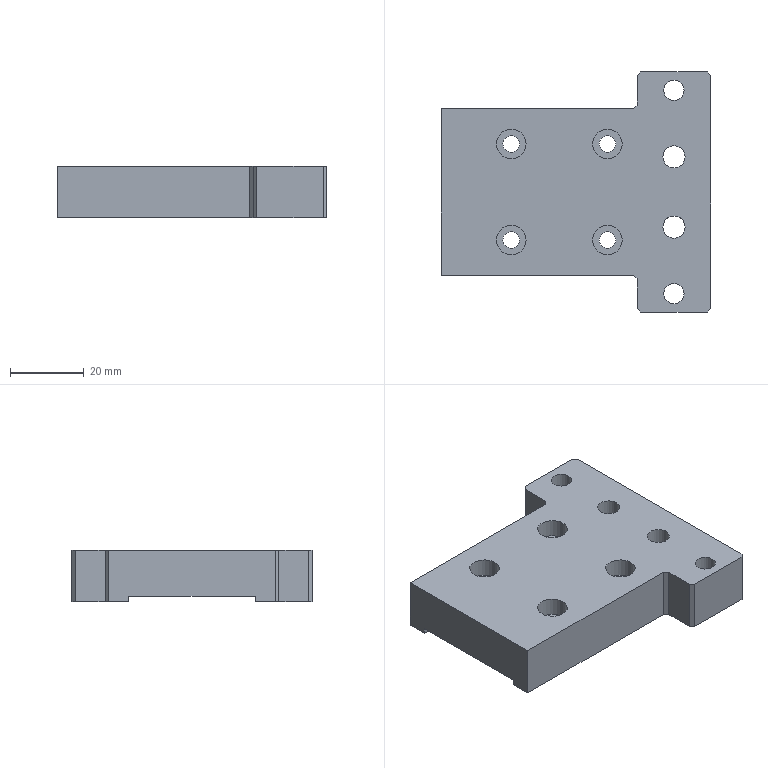Part | STEP file | Tube feed_id850_x_t | 1 solid | 40 faces | box 73 x 65 x 14 mm | volume 44658 mm3 | plane 26 | cylinder 14 | commonest cylinder face diameters 4.5 x4 8 x4 5.5 x2 6 x2 8.5 x2